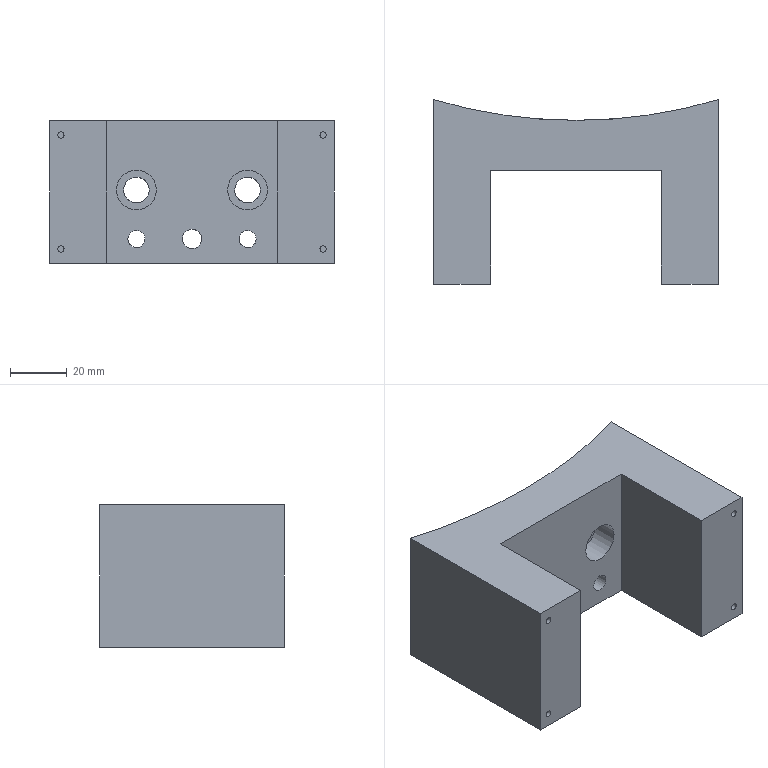NC program | NX | posted with a generic post | part box 100 x 64.77 x 50 mm
Whole program:
N10 G17 G21 G94 G90
(ZLEVEL_PROFILE_1_COPY , TOOL : D50R0.8)
N12 T02 M6
N14 G54
N16 G17 G0 G90 X107.699 Y74.397 B0. C0. S1200 M3
N18 G43 Z30. H2
N20 Z-0.5
N22 G94 G1 X100.344 Y72.638 F1500.
N24 G3 X96.714 Y69.2 R5.
N26 G1 X88.878 Y42.835
N28 X88.477 Y41.429
N30 G3 X87.076 Y36.198 R139.179
N32 X85.673 Y29.979 R141.946
N34 X84.271 Y22.012 R153.008
N36 X82.869 Y8.005 R149.38
N38 X82.869 Y-8.013 R147.41
N40 X84.272 Y-22.02 R149.442
N42 X85.675 Y-29.986 R153.286
N44 X87.077 Y-36.204 R142.694
N46 X88.478 Y-41.433 R138.543
N48 G1 X89.023 Y-43.319
N50 G3 X89.112 Y-43.625 R41.578
N52 G1 X96.714 Y-69.2
N54 G3 X100.344 Y-72.638 R5.
N56 G1 X107.699 Y-74.397
N58 G0 Z-1.
N60 G1 X100.344 Y-72.638
N62 G2 X96.714 Y-69.2 R5.
N64 G1 X88.878 Y-42.835
N66 G2 X88.878 Y42.835 R150.35
N68 G1 X96.714 Y69.2
N70 G2 X100.344 Y72.638 R5.
N72 G1 X107.699 Y74.397
N74 G0 Z-1.5
N76 G1 X100.344 Y72.638
N78 G3 X96.714 Y69.2 R5.
N80 G1 X88.878 Y42.835
N82 G3 X88.878 Y-42.835 R150.35
N84 G1 X96.714 Y-69.2
N86 G3 X100.344 Y-72.638 R5.
N88 G1 X107.699 Y-74.397
N90 G0 Z-2.
N92 G1 X100.344 Y-72.638
N94 G2 X96.714 Y-69.2 R5.
N96 G1 X88.878 Y-42.835
N98 G2 X88.878 Y42.835 R150.35
N100 G1 X96.714 Y69.2
N102 G2 X100.344 Y72.638 R5.
N104 G1 X107.699 Y74.397
N106 G0 Z-2.5
N108 G1 X100.344 Y72.638
N110 G3 X96.714 Y69.2 R5.
N112 G1 X88.878 Y42.835
N114 G3 X88.878 Y-42.835 R150.35
N116 G1 X96.714 Y-69.2
N118 G3 X100.344 Y-72.638 R5.
N120 G1 X107.699 Y-74.397
N122 G0 Z-3.
N124 G1 X100.344 Y-72.638
N126 G2 X96.714 Y-69.2 R5.
N128 G1 X88.878 Y-42.835
N130 G2 X88.878 Y42.835 R150.35
N132 G1 X96.714 Y69.2
N134 G2 X100.344 Y72.638 R5.
N136 G1 X107.699 Y74.397
N138 G0 Z-3.5
N140 G1 X100.344 Y72.638
N142 G3 X96.714 Y69.2 R5.
N144 G1 X88.878 Y42.835
N146 G3 X88.878 Y-42.835 R150.35
N148 G1 X96.714 Y-69.2
N150 G3 X100.344 Y-72.638 R5.
N152 G1 X107.699 Y-74.397
N154 G0 Z-4.
N156 G1 X100.344 Y-72.638
N158 G2 X96.714 Y-69.2 R5.
N160 G1 X88.878 Y-42.835
N162 G2 X88.878 Y42.835 R150.35
N164 G1 X96.714 Y69.2
N166 G2 X100.344 Y72.638 R5.
N168 G1 X107.699 Y74.397
N170 G0 Z-4.5
N172 G1 X100.344 Y72.638
N174 G3 X96.714 Y69.2 R5.
N176 G1 X88.878 Y42.835
N178 G3 X88.878 Y-42.835 R150.35
N180 G1 X96.714 Y-69.2
N182 G3 X100.344 Y-72.638 R5.
N184 G1 X107.699 Y-74.397
N186 G0 Z-5.
N188 G1 X100.344 Y-72.638
N190 G2 X96.714 Y-69.2 R5.
N192 G1 X88.878 Y-42.835
N194 G2 X88.878 Y42.835 R150.35
N196 G1 X96.714 Y69.2
N198 G2 X100.344 Y72.638 R5.
N200 G1 X107.699 Y74.397
N202 G0 Z-5.5
N204 G1 X100.344 Y72.638
N206 G3 X96.714 Y69.2 R5.
N208 G1 X88.878 Y42.835
N210 G3 X88.878 Y-42.835 R150.35
N212 G1 X96.714 Y-69.2
N214 G3 X100.344 Y-72.638 R5.
N216 G1 X107.699 Y-74.397
N218 G0 Z-6.
N220 G1 X100.344 Y-72.638
N222 G2 X96.714 Y-69.2 R5.
N224 G1 X88.878 Y-42.835
N226 G2 X88.878 Y42.835 R150.35
N228 G1 X96.714 Y69.2
N230 G2 X100.344 Y72.638 R5.
N232 G1 X107.699 Y74.397
N234 G0 Z-6.5
N236 G1 X100.344 Y72.638
N238 G3 X96.714 Y69.2 R5.
N240 G1 X88.878 Y42.835
N242 G3 X88.878 Y-42.835 R150.35
N244 G1 X96.714 Y-69.2
N246 G3 X100.344 Y-72.638 R5.
N248 G1 X107.699 Y-74.397
N250 G0 Z-7.
N252 G1 X100.344 Y-72.638
N254 G2 X96.714 Y-69.2 R5.
N256 G1 X88.878 Y-42.835
N258 G2 X88.878 Y42.835 R150.35
N260 G1 X96.714 Y69.2
N262 G2 X100.344 Y72.638 R5.
N264 G1 X107.699 Y74.397
N266 G0 Z-7.5
N268 G1 X100.344 Y72.638
N270 G3 X96.714 Y69.2 R5.
N272 G1 X88.878 Y42.835
N274 G3 X88.878 Y-42.835 R150.35
N276 G1 X96.714 Y-69.2
N278 G3 X100.344 Y-72.638 R5.
N280 G1 X107.699 Y-74.397
N282 G0 Z-8.
N284 G1 X100.344 Y-72.638
N286 G2 X96.714 Y-69.2 R5.
N288 G1 X88.878 Y-42.835
N290 G2 X88.878 Y42.835 R150.35
N292 G1 X96.714 Y69.2
N294 G2 X100.344 Y72.638 R5.
N296 G1 X107.699 Y74.397
N298 G0 Z-8.5
N300 G1 X100.344 Y72.638
N302 G3 X96.714 Y69.2 R5.
N304 G1 X88.878 Y42.835
N306 G3 X88.878 Y-42.835 R150.35
N308 G1 X96.714 Y-69.2
N310 G3 X100.344 Y-72.638 R5.
N312 G1 X107.699 Y-74.397
N314 G0 Z-9.
N316 G1 X100.344 Y-72.638
N318 G2 X96.714 Y-69.2 R5.
N320 G1 X88.878 Y-42.835
N322 G2 X88.878 Y42.835 R150.35
N324 G1 X96.714 Y69.2
N326 G2 X100.344 Y72.638 R5.
N328 G1 X107.699 Y74.397
N330 G0 Z-9.5
N332 G1 X100.344 Y72.638
N334 G3 X96.714 Y69.2 R5.
N336 G1 X88.878 Y42.835
N338 G3 X88.878 Y-42.835 R150.35
N340 G1 X96.714 Y-69.2
N342 G3 X100.344 Y-72.638 R5.
N344 G1 X107.699 Y-74.397
N346 G0 Z-10.
N348 G1 X100.344 Y-72.638
N350 G2 X96.714 Y-69.2 R5.
N352 G1 X88.878 Y-42.835
N354 G2 X88.878 Y42.835 R150.35
N356 G1 X96.714 Y69.2
N358 G2 X100.344 Y72.638 R5.
N360 G1 X107.699 Y74.397
N362 G0 Z-10.5
N364 G1 X100.344 Y72.638
N366 G3 X96.714 Y69.2 R5.
N368 G1 X88.878 Y42.835
N370 G3 X88.878 Y-42.835 R150.35
N372 G1 X96.714 Y-69.2
N374 G3 X100.344 Y-72.638 R5.
N376 G1 X107.699 Y-74.397
N378 G0 Z-11.
N380 G1 X100.344 Y-72.638
N382 G2 X96.714 Y-69.2 R5.
N384 G1 X88.878 Y-42.835
N386 G2 X88.878 Y42.835 R150.35
N388 G1 X96.714 Y69.2
N390 G2 X100.344 Y72.638 R5.
N392 G1 X107.699 Y74.397
N394 G0 Z-11.5
N396 G1 X100.344 Y72.638
N398 G3 X96.714 Y69.2 R5.
N400 G1 X88.878 Y42.835
N402 G3 X88.878 Y-42.835 R150.35
N404 G1 X96.714 Y-69.2
N406 G3 X100.344 Y-72.638 R5.
N408 G1 X107.699 Y-74.397
N410 G0 Z-12.
N412 G1 X100.344 Y-72.638
N414 G2 X96.714 Y-69.2 R5.
N416 G1 X88.878 Y-42.835
N418 G2 X88.878 Y42.835 R150.35
N420 G1 X96.714 Y69.2
N422 G2 X100.344 Y72.638 R5.
N424 G1 X107.699 Y74.397
N426 G0 Z-12.5
N428 G1 X100.344 Y72.638
N430 G3 X96.714 Y69.2 R5.
N432 G1 X88.878 Y42.835
N434 G3 X88.878 Y-42.835 R150.35
N436 G1 X96.714 Y-69.2
N438 G3 X100.344 Y-72.638 R5.
N440 G1 X107.699 Y-74.397
N442 G0 Z-13.
N444 G1 X100.344 Y-72.638
N446 G2 X96.714 Y-69.2 R5.
N448 G1 X88.878 Y-42.835
N450 G2 X88.878 Y42.835 R150.35
N452 G1 X96.714 Y69.2
N454 G2 X100.344 Y72.638 R5.
N456 G1 X107.699 Y74.397
N458 G0 Z-13.5
N460 G1 X100.344 Y72.638
N462 G3 X96.714 Y69.2 R5.
N464 G1 X88.878 Y42.835
N466 G3 X88.878 Y-42.835 R150.35
N468 G1 X96.714 Y-69.2
N470 G3 X100.344 Y-72.638 R5.
N472 G1 X107.699 Y-74.397
N474 G0 Z-14.
N476 G1 X100.344 Y-72.638
N478 G2 X96.714 Y-69.2 R5.
N480 G1 X88.878 Y-42.835
N482 G2 X88.878 Y42.835 R150.35
N484 G1 X96.714 Y69.2
N486 G2 X100.344 Y72.638 R5.
N488 G1 X107.699 Y74.397
N490 G0 Z-14.5
N492 G1 X100.344 Y72.638
N494 G3 X96.714 Y69.2 R5.
N496 G1 X88.878 Y42.835
N498 G3 X88.878 Y-42.835 R150.35
N500 G1 X96.714 Y-69.2
N502 G3 X100.344 Y-72.638 R5.
N504 G1 X107.699 Y-74.397
N506 G0 Z-15.
N508 G1 X100.344 Y-72.638
N510 G2 X96.714 Y-69.2 R5.
N512 G1 X88.878 Y-42.835
N514 G2 X88.878 Y42.835 R150.35
N516 G1 X96.714 Y69.2
N518 G2 X100.344 Y72.638 R5.
N520 G1 X107.699 Y74.397
N522 G0 Z-15.5
N524 G1 X100.344 Y72.638
N526 G3 X96.714 Y69.2 R5.
N528 G1 X88.878 Y42.835
N530 G3 X88.878 Y-42.835 R150.35
N532 G1 X96.714 Y-69.2
N534 G3 X100.344 Y-72.638 R5.
N536 G1 X107.699 Y-74.397
N538 G0 Z-16.
N540 G1 X100.344 Y-72.638
N542 G2 X96.714 Y-69.2 R5.
N544 G1 X88.878 Y-42.835
N546 G2 X88.878 Y42.835 R150.35
N548 G1 X96.714 Y69.2
N550 G2 X100.344 Y72.638 R5.
N552 G1 X107.699 Y74.397
N554 G0 Z-16.5
N556 G1 X100.344 Y72.638
N558 G3 X96.714 Y69.2 R5.
N560 G1 X88.878 Y42.835
N562 G3 X88.878 Y-42.835 R150.35
N564 G1 X96.714 Y-69.2
N566 G3 X100.344 Y-72.638 R5.
N568 G1 X107.699 Y-74.397
N570 G0 Z-17.
N572 G1 X100.344 Y-72.638
N574 G2 X96.714 Y-69.2 R5.
N576 G1 X88.878 Y-42.835
N578 G2 X88.878 Y42.835 R150.35
N580 G1 X96.714 Y69.2
N582 G2 X100.344 Y72.638 R5.
N584 G1 X107.699 Y74.397
N586 G0 Z-17.5
N588 G1 X100.344 Y72.638
N590 G3 X96.714 Y69.2 R5.
N592 G1 X88.878 Y42.835
N594 G3 X88.878 Y-42.835 R150.35
N596 G1 X96.714 Y-69.2
N598 G3 X100.344 Y-72.638 R5.
N600 G1 X107.699 Y-74.397
N602 G0 Z-18.
N604 G1 X100.344 Y-72.638
N606 G2 X96.714 Y-69.2 R5.
N608 G1 X88.878 Y-42.835
N610 G2 X88.878 Y42.835 R150.35
N612 G1 X96.714 Y69.2
N614 G2 X100.344 Y72.638 R5.
N616 G1 X107.699 Y74.397
N618 G0 Z-18.5
N620 G1 X100.344 Y72.638
N622 G3 X96.714 Y69.2 R5.
N624 G1 X88.878 Y42.835
N626 G3 X88.878 Y-42.835 R150.35
N628 G1 X96.714 Y-69.2
N630 G3 X100.344 Y-72.638 R5.
N632 G1 X107.699 Y-74.397
N634 G0 Z-19.
N636 G1 X100.344 Y-72.638
N638 G2 X96.714 Y-69.2 R5.
N640 G1 X88.878 Y-42.835
N642 G2 X88.878 Y42.835 R150.35
N644 G1 X96.714 Y69.2
N646 G2 X100.344 Y72.638 R5.
N648 G1 X107.699 Y74.397
N650 G0 Z-19.5
N652 G1 X100.344 Y72.638
N654 G3 X96.714 Y69.2 R5.
N656 G1 X88.878 Y42.835
N658 G3 X88.878 Y-42.835 R150.35
N660 G1 X96.714 Y-69.2
N662 G3 X100.344 Y-72.638 R5.
N664 G1 X107.699 Y-74.397
N666 G0 Z-20.
N668 G1 X100.344 Y-72.638
N670 G2 X96.714 Y-69.2 R5.
N672 G1 X88.878 Y-42.835
N674 G2 X88.878 Y42.835 R150.35
N676 G1 X96.714 Y69.2
N678 G2 X100.344 Y72.638 R5.
N680 G1 X107.699 Y74.397
N682 G0 Z-20.5
N684 G1 X100.344 Y72.638
N686 G3 X96.714 Y69.2 R5.
N688 G1 X88.878 Y42.835
N690 G3 X88.878 Y-42.835 R150.35
N692 G1 X96.714 Y-69.2
N694 G3 X100.344 Y-72.638 R5.
N696 G1 X107.699 Y-74.397
N698 G0 Z-21.
N700 G1 X100.344 Y-72.638
N702 G2 X96.714 Y-69.2 R5.
N704 G1 X88.878 Y-42.835
N706 G2 X88.878 Y42.835 R150.35
N708 G1 X96.714 Y69.2
N710 G2 X100.344 Y72.638 R5.
N712 G1 X107.699 Y74.397
N714 G0 Z-21.5
N716 G1 X100.344 Y72.638
N718 G3 X96.714 Y69.2 R5.
N720 G1 X88.878 Y42.835
N722 G3 X88.878 Y-42.835 R150.35
N724 G1 X96.714 Y-69.2
N726 G3 X100.344 Y-72.638 R5.
N728 G1 X107.699 Y-74.397
N730 G0 Z-22.
N732 G1 X100.344 Y-72.638
N734 G2 X96.714 Y-69.2 R5.
N736 G1 X88.878 Y-42.835
N738 G2 X88.878 Y42.835 R150.35
N740 G1 X96.714 Y69.2
N742 G2 X100.344 Y72.638 R5.
N744 G1 X107.699 Y74.397
N746 G0 Z-22.5
N748 G1 X100.344 Y72.638
N750 G3 X96.714 Y69.2 R5.
N752 G1 X88.878 Y42.835
N754 G3 X88.878 Y-42.835 R150.35
N756 G1 X96.714 Y-69.2
N758 G3 X100.344 Y-72.638 R5.
N760 G1 X107.699 Y-74.397
N762 G0 Z-23.
N764 G1 X100.344 Y-72.638
N766 G2 X96.714 Y-69.2 R5.
N768 G1 X88.878 Y-42.835
N770 G2 X88.878 Y42.835 R150.35
N772 G1 X96.714 Y69.2
N774 G2 X100.344 Y72.638 R5.
N776 G1 X107.699 Y74.397
N778 G0 Z-23.5
N780 G1 X100.344 Y72.638
N782 G3 X96.714 Y69.2 R5.
N784 G1 X88.878 Y42.835
N786 G3 X88.878 Y-42.835 R150.35
N788 G1 X96.714 Y-69.2
N790 G3 X100.344 Y-72.638 R5.
N792 G1 X107.699 Y-74.397
N794 G0 Z-24.
N796 G1 X100.344 Y-72.638
N798 G2 X96.714 Y-69.2 R5.
N800 G1 X88.878 Y-42.835
N802 G2 X88.878 Y42.835 R150.35
N804 G1 X96.714 Y69.2
N806 G2 X100.344 Y72.638 R5.
N808 G1 X107.699 Y74.397
N810 G0 Z-24.5
N812 G1 X100.344 Y72.638
N814 G3 X96.714 Y69.2 R5.
N816 G1 X88.878 Y42.835
N818 G3 X88.878 Y-42.835 R150.35
N820 G1 X96.714 Y-69.2
N822 G3 X100.344 Y-72.638 R5.
N824 G1 X107.699 Y-74.397
N826 G0 Z-25.
N828 G1 X100.344 Y-72.638
N830 G2 X96.714 Y-69.2 R5.
N832 G1 X88.878 Y-42.835
N834 G2 X88.878 Y42.835 R150.35
N836 G1 X96.714 Y69.2
N838 G2 X100.344 Y72.638 R5.
N840 G1 X107.699 Y74.397
N842 G0 Z-25.5
N844 G1 X100.344 Y72.638
N846 G3 X96.714 Y69.2 R5.
N848 G1 X88.878 Y42.835
N850 G3 X88.878 Y-42.835 R150.35
N852 G1 X96.714 Y-69.2
N854 G3 X100.344 Y-72.638 R5.
N856 G1 X107.699 Y-74.397
N858 G0 Z-26.
N860 G1 X100.344 Y-72.638
N862 G2 X96.714 Y-69.2 R5.
N864 G1 X88.878 Y-42.835
N866 G2 X88.878 Y42.835 R150.35
N868 G1 X96.714 Y69.2
N870 G2 X100.344 Y72.638 R5.
N872 G1 X107.699 Y74.397
N874 G0 Z-26.5
N876 G1 X100.344 Y72.638
N878 G3 X96.714 Y69.2 R5.
N880 G1 X88.878 Y42.835
N882 G3 X88.878 Y-42.835 R150.35
N884 G1 X96.714 Y-69.2
N886 G3 X100.344 Y-72.638 R5.
N888 G1 X107.699 Y-74.397
N890 G0 Z-27.
N892 G1 X100.344 Y-72.638
N894 G2 X96.714 Y-69.2 R5.
N896 G1 X88.878 Y-42.835
N898 G2 X88.878 Y42.835 R150.35
N900 G1 X96.714 Y69.2
N902 G2 X100.344 Y72.638 R5.
N904 G1 X107.699 Y74.397
N906 G0 Z-27.5
N908 G1 X100.344 Y72.638
N910 G3 X96.714 Y69.2 R5.
N912 G1 X88.878 Y42.835
N914 G3 X88.878 Y-42.835 R150.35
N916 G1 X96.714 Y-69.2
N918 G3 X100.344 Y-72.638 R5.
N920 G1 X107.699 Y-74.397
N922 G0 Z-28.
N924 G1 X100.344 Y-72.638
N926 G2 X96.714 Y-69.2 R5.
N928 G1 X88.878 Y-42.835
N930 G2 X88.878 Y42.835 R150.35
N932 G1 X96.714 Y69.2
N934 G2 X100.344 Y72.638 R5.
N936 G1 X107.699 Y74.397
N938 G0 Z-28.5
N940 G1 X100.344 Y72.638
N942 G3 X96.714 Y69.2 R5.
N944 G1 X88.878 Y42.835
N946 G3 X88.878 Y-42.835 R150.35
N948 G1 X96.714 Y-69.2
N950 G3 X100.344 Y-72.638 R5.
N952 G1 X107.699 Y-74.397
N954 G0 Z-29.
N956 G1 X100.344 Y-72.638
N958 G2 X96.714 Y-69.2 R5.
N960 G1 X88.878 Y-42.835
N962 G2 X88.878 Y42.835 R150.35
N964 G1 X96.714 Y69.2
N966 G2 X100.344 Y72.638 R5.
N968 G1 X107.699 Y74.397
N970 G0 Z-29.5
N972 G1 X100.344 Y72.638
N974 G3 X96.714 Y69.2 R5.
N976 G1 X88.878 Y42.835
N978 G3 X88.878 Y-42.835 R150.35
N980 G1 X96.714 Y-69.2
N982 G3 X100.344 Y-72.638 R5.
N984 G1 X107.699 Y-74.397
N986 G0 Z-30.
N988 G1 X100.344 Y-72.638
N990 G2 X96.714 Y-69.2 R5.
N992 G1 X88.878 Y-42.835
N994 G2 X88.878 Y42.835 R150.35
N996 G1 X96.714 Y69.2
N998 G2 X100.344 Y72.638 R5.
N1000 G1 X107.699 Y74.397
N1002 G0 Z-30.5
N1004 G1 X100.344 Y72.638
N1006 G3 X96.714 Y69.2 R5.
N1008 G1 X88.878 Y42.835
N1010 G3 X88.878 Y-42.835 R150.35
N1012 G1 X96.714 Y-69.2
N1014 G3 X100.344 Y-72.638 R5.
N1016 G1 X107.699 Y-74.397
N1018 G0 Z-31.
N1020 G1 X100.344 Y-72.638
N1022 G2 X96.714 Y-69.2 R5.
N1024 G1 X88.878 Y-42.835
N1026 G2 X88.878 Y42.835 R150.35
N1028 G1 X96.714 Y69.2
N1030 G2 X100.344 Y72.638 R5.
N1032 G1 X107.699 Y74.397
N1034 G0 Z-31.5
N1036 G1 X100.344 Y72.638
N1038 G3 X96.714 Y69.2 R5.
N1040 G1 X88.878 Y42.835
N1042 G3 X88.878 Y-42.835 R150.35
N1044 G1 X96.714 Y-69.2
N1046 G3 X100.344 Y-72.638 R5.
N1048 G1 X107.699 Y-74.397
N1050 G0 Z-32.
N1052 G1 X100.344 Y-72.638
N1054 G2 X96.714 Y-69.2 R5.
N1056 G1 X88.878 Y-42.835
N1058 G2 X88.878 Y42.835 R150.35
N1060 G1 X96.714 Y69.2
N1062 G2 X100.344 Y72.638 R5.
N1064 G1 X107.699 Y74.397
N1066 G0 Z-32.5
N1068 G1 X100.344 Y72.638
N1070 G3 X96.714 Y69.2 R5.
N1072 G1 X88.878 Y42.835
N1074 G3 X88.878 Y-42.835 R150.35
N1076 G1 X96.714 Y-69.2
N1078 G3 X100.344 Y-72.638 R5.
N1080 G1 X107.699 Y-74.397
N1082 G0 Z-33.
N1084 G1 X100.344 Y-72.638
N1086 G2 X96.714 Y-69.2 R5.
N1088 G1 X88.878 Y-42.835
N1090 G2 X88.878 Y42.835 R150.35
N1092 G1 X96.714 Y69.2
N1094 G2 X100.344 Y72.638 R5.
N1096 G1 X107.699 Y74.397
N1098 G0 Z-33.5
N1100 G1 X100.344 Y72.638
N1102 G3 X96.714 Y69.2 R5.
N1104 G1 X88.878 Y42.835
N1106 G3 X88.878 Y-42.835 R150.35
N1108 G1 X96.714 Y-69.2
N1110 G3 X100.344 Y-72.638 R5.
N1112 G1 X107.699 Y-74.397
N1114 G0 Z-34.
N1116 G1 X100.344 Y-72.638
N1118 G2 X96.714 Y-69.2 R5.
N1120 G1 X88.878 Y-42.835
N1122 G2 X88.878 Y42.835 R150.35
N1124 G1 X96.714 Y69.2
N1126 G2 X100.344 Y72.638 R5.
N1128 G1 X107.699 Y74.397
N1130 G0 Z-34.5
N1132 G1 X100.344 Y72.638
N1134 G3 X96.714 Y69.2 R5.
N1136 G1 X88.878 Y42.835
N1138 G3 X88.878 Y-42.835 R150.35
N1140 G1 X96.714 Y-69.2
N1142 G3 X100.344 Y-72.638 R5.
N1144 G1 X107.699 Y-74.397
N1146 G0 Z-35.
N1148 G1 X100.344 Y-72.638
N1150 G2 X96.714 Y-69.2 R5.
N1152 G1 X88.878 Y-42.835
N1154 G2 X88.878 Y42.835 R150.35
N1156 G1 X96.714 Y69.2
N1158 G2 X100.344 Y72.638 R5.
N1160 G1 X107.699 Y74.397
N1162 G0 Z-35.5
N1164 G1 X100.344 Y72.638
N1166 G3 X96.714 Y69.2 R5.
N1168 G1 X88.878 Y42.835
N1170 G3 X88.878 Y-42.835 R150.35
N1172 G1 X96.714 Y-69.2
N1174 G3 X100.344 Y-72.638 R5.
N1176 G1 X107.699 Y-74.397
N1178 G0 Z-36.
N1180 G1 X100.344 Y-72.638
N1182 G2 X96.714 Y-69.2 R5.
N1184 G1 X88.878 Y-42.835
N1186 G2 X88.878 Y42.835 R150.35
N1188 G1 X96.714 Y69.2
N1190 G2 X100.344 Y72.638 R5.
N1192 G1 X107.699 Y74.397
N1194 G0 Z-36.5
N1196 G1 X100.344 Y72.638
N1198 G3 X96.714 Y69.2 R5.
N1200 G1 X88.878 Y42.835
N1202 G3 X88.878 Y-42.835 R150.35
N1204 G1 X96.714 Y-69.2
N1206 G3 X100.344 Y-72.638 R5.
N1208 G1 X107.699 Y-74.397
N1210 G0 Z-37.
N1212 G1 X100.344 Y-72.638
N1214 G2 X96.714 Y-69.2 R5.
N1216 G1 X88.878 Y-42.835
N1218 G2 X88.878 Y42.835 R150.35
N1220 G1 X96.714 Y69.2
N1222 G2 X100.344 Y72.638 R5.
N1224 G1 X107.699 Y74.397
N1226 G0 Z-37.5
N1228 G1 X100.344 Y72.638
N1230 G3 X96.714 Y69.2 R5.
N1232 G1 X88.878 Y42.835
N1234 G3 X88.878 Y-42.835 R150.35
N1236 G1 X96.714 Y-69.2
N1238 G3 X100.344 Y-72.638 R5.
N1240 G1 X107.699 Y-74.397
N1242 G0 Z-38.
N1244 G1 X100.344 Y-72.638
N1246 G2 X96.714 Y-69.2 R5.
N1248 G1 X88.878 Y-42.835
N1250 G2 X88.878 Y42.835 R150.35
N1252 G1 X96.714 Y69.2
N1254 G2 X100.344 Y72.638 R5.
N1256 G1 X107.699 Y74.397
N1258 G0 Z-38.5
N1260 G1 X100.344 Y72.638
N1262 G3 X96.714 Y69.2 R5.
N1264 G1 X88.878 Y42.835
N1266 G3 X88.878 Y-42.835 R150.35
N1268 G1 X96.714 Y-69.2
N1270 G3 X100.344 Y-72.638 R5.
N1272 G1 X107.699 Y-74.397
N1274 G0 Z-39.
N1276 G1 X100.344 Y-72.638
N1278 G2 X96.714 Y-69.2 R5.
N1280 G1 X88.878 Y-42.835
N1282 G2 X88.878 Y42.835 R150.35
N1284 G1 X96.714 Y69.2
N1286 G2 X100.344 Y72.638 R5.
N1288 G1 X107.699 Y74.397
N1290 G0 Z-39.5
N1292 G1 X100.344 Y72.638
N1294 G3 X96.714 Y69.2 R5.
N1296 G1 X88.878 Y42.835
N1298 G3 X88.878 Y-42.835 R150.35
N1300 G1 X96.714 Y-69.2
N1302 G3 X100.344 Y-72.638 R5.
N1304 G1 X107.699 Y-74.397
N1306 G0 Z-40.
N1308 G1 X100.344 Y-72.638
N1310 G2 X96.714 Y-69.2 R5.
N1312 G1 X88.878 Y-42.835
N1314 G2 X88.878 Y42.835 R150.35
N1316 G1 X96.714 Y69.2
N1318 G2 X100.344 Y72.638 R5.
N1320 G1 X107.699 Y74.397
N1322 G0 Z-40.5
N1324 G1 X100.344 Y72.638
N1326 G3 X96.714 Y69.2 R5.
N1328 G1 X88.878 Y42.835
N1330 G3 X88.878 Y-42.835 R150.35
N1332 G1 X96.714 Y-69.2
N1334 G3 X100.344 Y-72.638 R5.
N1336 G1 X107.699 Y-74.397
N1338 G0 Z-41.
N1340 G1 X100.344 Y-72.638
N1342 G2 X96.714 Y-69.2 R5.
N1344 G1 X88.878 Y-42.835
N1346 G2 X88.878 Y42.835 R150.35
N1348 G1 X96.714 Y69.2
N1350 G2 X100.344 Y72.638 R5.
N1352 G1 X107.699 Y74.397
N1354 G0 Z-41.5
N1356 G1 X100.344 Y72.638
N1358 G3 X96.714 Y69.2 R5.
N1360 G1 X88.878 Y42.835
N1362 G3 X88.878 Y-42.835 R150.35
N1364 G1 X96.714 Y-69.2
N1366 G3 X100.344 Y-72.638 R5.
N1368 G1 X107.699 Y-74.397
N1370 G0 Z-42.
N1372 G1 X100.344 Y-72.638
N1374 G2 X96.714 Y-69.2 R5.
N1376 G1 X88.878 Y-42.835
N1378 G2 X88.878 Y42.835 R150.35
N1380 G1 X96.714 Y69.2
N1382 G2 X100.344 Y72.638 R5.
N1384 G1 X107.699 Y74.397
N1386 G0 Z-42.5
N1388 G1 X100.344 Y72.638
N1390 G3 X96.714 Y69.2 R5.
N1392 G1 X88.878 Y42.835
N1394 G3 X88.878 Y-42.835 R150.35
N1396 G1 X96.714 Y-69.2
N1398 G3 X100.344 Y-72.638 R5.
N1400 G1 X107.699 Y-74.397
N1402 G0 Z-43.
N1404 G1 X100.344 Y-72.638
N1406 G2 X96.714 Y-69.2 R5.
N1408 G1 X88.878 Y-42.835
N1410 G2 X88.878 Y42.835 R150.35
N1412 G1 X96.714 Y69.2
N1414 G2 X100.344 Y72.638 R5.
N1416 G1 X107.699 Y74.397
N1418 G0 Z-43.5
N1420 G1 X100.344 Y72.638
N1422 G3 X96.714 Y69.2 R5.
N1424 G1 X88.878 Y42.835
N1426 G3 X88.878 Y-42.835 R150.35
N1428 G1 X96.714 Y-69.2
N1430 G3 X100.344 Y-72.638 R5.
N1432 G1 X107.699 Y-74.397
N1434 G0 Z-44.
N1436 G1 X100.344 Y-72.638
N1438 G2 X96.714 Y-69.2 R5.
N1440 G1 X88.878 Y-42.835
N1442 G2 X88.878 Y42.835 R150.35
N1444 G1 X96.714 Y69.2
N1446 G2 X100.344 Y72.638 R5.
N1448 G1 X107.699 Y74.397
N1450 G0 Z-44.5
N1452 G1 X100.344 Y72.638
N1454 G3 X96.714 Y69.2 R5.
N1456 G1 X88.878 Y42.835
N1458 G3 X88.878 Y-42.835 R150.35
N1460 G1 X96.714 Y-69.2
N1462 G3 X100.344 Y-72.638 R5.
N1464 G1 X107.699 Y-74.397
N1466 G0 Z-45.
N1468 G1 X100.344 Y-72.638
N1470 G2 X96.714 Y-69.2 R5.
N1472 G1 X88.878 Y-42.835
N1474 G2 X88.878 Y42.835 R150.35
N1476 G1 X96.714 Y69.2
N1478 G2 X100.344 Y72.638 R5.
N1480 G1 X107.699 Y74.397
N1482 G0 Z-45.5
N1484 G1 X100.344 Y72.638
N1486 G3 X96.714 Y69.2 R5.
N1488 G1 X88.878 Y42.835
N1490 G3 X88.878 Y-42.835 R150.35
N1492 G1 X96.714 Y-69.2
N1494 G3 X100.344 Y-72.638 R5.
N1496 G1 X107.699 Y-74.397
N1498 G0 Z-46.
N1500 G1 X100.344 Y-72.638
N1502 G2 X96.714 Y-69.2 R5.
N1504 G1 X88.878 Y-42.835
N1506 G2 X88.878 Y42.835 R150.35
N1508 G1 X96.714 Y69.2
N1510 G2 X100.344 Y72.638 R5.
N1512 G1 X107.699 Y74.397
N1514 G0 Z-46.5
N1516 G1 X100.344 Y72.638
N1518 G3 X96.714 Y69.2 R5.
N1520 G1 X88.878 Y42.835
N1522 G3 X88.878 Y-42.835 R150.35
N1524 G1 X96.714 Y-69.2
N1526 G3 X100.344 Y-72.638 R5.
N1528 G1 X107.699 Y-74.397
N1530 G0 Z-47.
N1532 G1 X100.344 Y-72.638
N1534 G2 X96.714 Y-69.2 R5.
N1536 G1 X88.878 Y-42.835
N1538 G2 X88.878 Y42.835 R150.35
N1540 G1 X96.714 Y69.2
N1542 G2 X100.344 Y72.638 R5.
N1544 G1 X107.699 Y74.397
N1546 G0 Z-47.5
N1548 G1 X100.344 Y72.638
N1550 G3 X96.714 Y69.2 R5.
N1552 G1 X88.878 Y42.835
N1554 G3 X88.878 Y-42.835 R150.35
N1556 G1 X96.714 Y-69.2
N1558 G3 X100.344 Y-72.638 R5.
N1560 G1 X107.699 Y-74.397
N1562 G0 Z-48.
N1564 G1 X100.344 Y-72.638
N1566 G2 X96.714 Y-69.2 R5.
N1568 G1 X88.878 Y-42.835
N1570 G2 X88.878 Y42.835 R150.35
N1572 G1 X96.714 Y69.2
N1574 G2 X100.344 Y72.638 R5.
N1576 G1 X107.699 Y74.397
N1578 G0 Z-48.5
N1580 G1 X100.344 Y72.638
N1582 G3 X96.714 Y69.2 R5.
N1584 G1 X88.878 Y42.835
N1586 G3 X88.878 Y-42.835 R150.35
N1588 G1 X96.714 Y-69.2
N1590 G3 X100.344 Y-72.638 R5.
N1592 G1 X107.699 Y-74.397
N1594 G0 Z-49.
N1596 G1 X100.344 Y-72.638
N1598 G2 X96.714 Y-69.2 R5.
N1600 G1 X88.878 Y-42.835
N1602 G2 X88.878 Y42.835 R150.35
N1604 G1 X96.714 Y69.2
N1606 G2 X100.344 Y72.638 R5.
N1608 G1 X107.699 Y74.397
N1610 G0 Z-49.5
N1612 G1 X100.344 Y72.638
N1614 G3 X96.714 Y69.2 R5.
N1616 G1 X88.878 Y42.835
N1618 G3 X88.878 Y-42.835 R150.35
N1620 G1 X96.714 Y-69.2
N1622 G3 X100.344 Y-72.638 R5.
N1624 G1 X107.699 Y-74.397
N1626 G0 Z-50.
N1628 G1 X100.344 Y-72.638
N1630 G2 X96.714 Y-69.2 R5.
N1632 G1 X88.878 Y-42.835
N1634 G2 X88.878 Y42.835 R150.35
N1636 G1 X96.714 Y69.2
N1638 G2 X100.344 Y72.638 R5.
N1640 G1 X107.699 Y74.397
N1642 G0 Z-50.5
N1644 G1 X100.344 Y72.638
N1646 G3 X96.714 Y69.2 R5.
N1648 G1 X88.878 Y42.835
N1650 G3 X88.878 Y-42.835 R150.35
N1652 G1 X96.714 Y-69.2
N1654 G3 X100.344 Y-72.638 R5.
N1656 G1 X107.699 Y-74.397
N1658 G0 Z-51.
N1660 G1 X100.344 Y-72.638
N1662 G2 X96.714 Y-69.2 R5.
N1664 G1 X88.878 Y-42.835
N1666 G2 X88.878 Y42.835 R150.35
N1668 G1 X96.714 Y69.2
N1670 G2 X100.344 Y72.638 R5.
N1672 G1 X107.699 Y74.397
N1674 G0 Z30.
N1676 M5
(11_COPY , TOOL : D10JING)
N1678 T11 M6
N1680 G54
N1682 G17 G0 G90 X72.289 Y54.507 B0. C0. S5500 M3
N1684 G43 Z30. H11
N1686 Z-14.
N1688 G94 G1 Z-15. F1000.
N1690 X71.813 Y54.393
N1692 G3 X71.087 Y53.706 R1.
N1694 G1 X69.566 Y48.586
N1696 G3 X69.563 Y-48.575 R170.5
N1698 G1 X69.675 Y-49.029
N1700 X69.698 Y-49.039
N1702 X71.087 Y-53.706
N1704 G3 X71.813 Y-54.393 R1.
N1706 G1 X72.289 Y-54.507
N1708 Z-14.
N1710 G0 Y54.507 Z-25.667
N1712 G1 Z-26.667
N1714 X71.813 Y54.393
N1716 G3 X71.087 Y53.706 R1.
N1718 G1 X69.566 Y48.586
N1720 G3 X69.563 Y-48.575 R170.5
N1722 G1 X69.675 Y-49.029
N1724 X69.699 Y-49.039
N1726 X71.087 Y-53.706
N1728 G3 X71.813 Y-54.393 R1.
N1730 G1 X72.289 Y-54.507
N1732 Z-25.667
N1734 G0 X72.29 Y54.507 Z-37.333
N1736 G1 Z-38.333
N1738 X71.813 Y54.393
N1740 G3 X71.087 Y53.705 R1.
N1742 G1 X69.566 Y48.586
N1744 G3 X69.563 Y-48.575 R170.5
N1746 G1 X69.675 Y-49.029
N1748 X69.7 Y-49.039
N1750 X71.087 Y-53.706
N1752 G3 X71.813 Y-54.393 R1.
N1754 G1 X72.289 Y-54.507
N1756 Z-37.333
N1758 G0 X72.29 Y54.507 Z-49.
N1760 G1 Z-50.
N1762 X71.813 Y54.393
N1764 G3 X71.087 Y53.705 R1.
N1766 G1 X69.566 Y48.586
N1768 G3 X69.563 Y-48.575 R170.5
N1770 G1 X69.672 Y-49.015
N1772 X69.69 Y-49.008
N1774 X69.704 Y-49.02
N1776 X69.7 Y-49.039
N1778 X71.087 Y-53.706
N1780 G3 X71.813 Y-54.393 R1.
N1782 G1 X72.29 Y-54.507
N1784 Z-49.
N1786 G0 Z30.
N1788 M5
N1790 M2